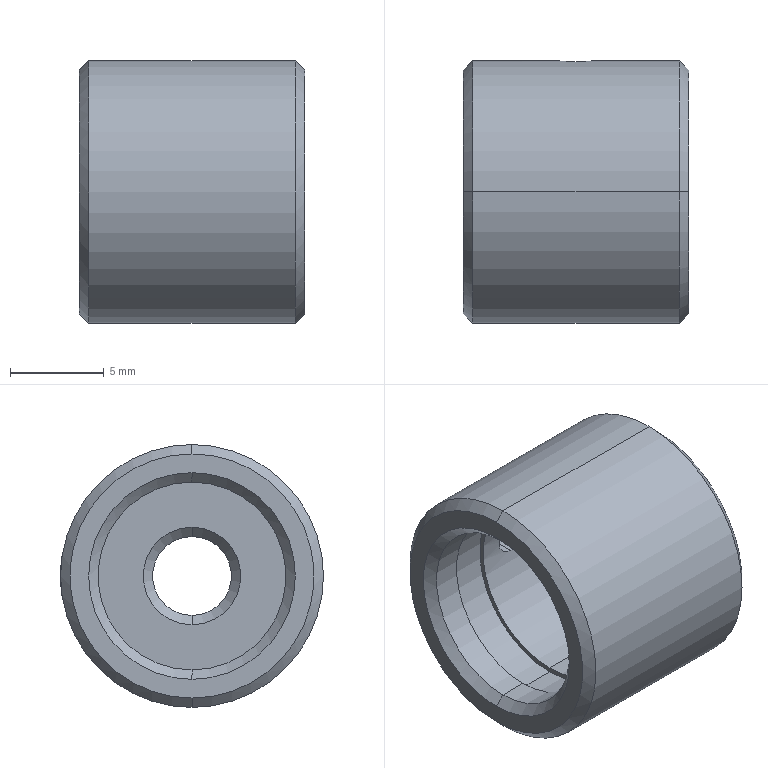Part | SolidWorks | features BaseBody 1 | 1 solid | 27 faces | box 12 x 14 x 14 mm | volume 997.34 mm3 | cylinder 12 | cone 10 | plane 5 | commonest cylinder face diameters 10 x4 1.6 x2 4.2 x2 10.5 x2 14 x2
STEP:
#1=CARTESIAN_POINT('',(-6.,6.934,0.959));
#2=VERTEX_POINT('',#1);
#3=CARTESIAN_POINT('',(-6.,6.934,-0.959));
#4=VERTEX_POINT('',#3);
#5=CARTESIAN_POINT('',(-6.,6.934,0.959));
#6=CARTESIAN_POINT('',(-6.131,6.934,0.959));
#7=CARTESIAN_POINT('',(-6.259,6.937,0.9359));
#8=CARTESIAN_POINT('',(-6.503,6.949,0.844));
#9=CARTESIAN_POINT('',(-6.615,6.957,0.7765));
#10=CARTESIAN_POINT('',(-6.808,6.975,0.6024));
#11=CARTESIAN_POINT('',(-6.887,6.983,0.4966));
#12=CARTESIAN_POINT('',(-6.996,6.996,0.2614));
#13=CARTESIAN_POINT('',(-7.025,7.,0.1312));
#14=CARTESIAN_POINT('',(-7.025,7.,-0.1276));
#15=CARTESIAN_POINT('',(-6.997,6.996,-0.258));
#16=CARTESIAN_POINT('',(-6.889,6.984,-0.4943));
#17=CARTESIAN_POINT('',(-6.81,6.975,-0.6004));
#18=CARTESIAN_POINT('',(-6.519,6.949,-0.8639));
#19=CARTESIAN_POINT('',(-6.262,6.934,-0.959));
#20=CARTESIAN_POINT('',(-6.,6.934,-0.959));
#21=B_SPLINE_CURVE_WITH_KNOTS('',3,(#5,#6,#7,#8,#9,#10,#11,#12,#13,#14,#15,#16,#17,#18,#19,#20),.UNSPECIFIED.,.F.,.F.,(4,2,2,2,2,2,2,4),(0.,0.0003877,0.0007754,0.001163,0.001551,0.001938,0.002326,0.003101),.UNSPECIFIED.);
#22=EDGE_CURVE('',#2,#4,#21,.T.);
#23=ORIENTED_EDGE('',*,*,#22,.T.);
#24=CARTESIAN_POINT('',(-6.,6.934,-0.959));
#25=CARTESIAN_POINT('',(-5.869,6.934,-0.959));
#26=CARTESIAN_POINT('',(-5.741,6.937,-0.9359));
#27=CARTESIAN_POINT('',(-5.497,6.949,-0.844));
#28=CARTESIAN_POINT('',(-5.385,6.957,-0.7765));
#29=CARTESIAN_POINT('',(-5.192,6.975,-0.6024));
#30=CARTESIAN_POINT('',(-5.113,6.983,-0.4966));
#31=CARTESIAN_POINT('',(-5.004,6.996,-0.2614));
#32=CARTESIAN_POINT('',(-4.975,7.,-0.1312));
#33=CARTESIAN_POINT('',(-4.975,7.,0.1276));
#34=CARTESIAN_POINT('',(-5.003,6.996,0.258));
#35=CARTESIAN_POINT('',(-5.111,6.984,0.4943));
#36=CARTESIAN_POINT('',(-5.19,6.975,0.6004));
#37=CARTESIAN_POINT('',(-5.481,6.949,0.8639));
#38=CARTESIAN_POINT('',(-5.738,6.934,0.959));
#39=CARTESIAN_POINT('',(-6.,6.934,0.959));
#40=B_SPLINE_CURVE_WITH_KNOTS('',3,(#24,#25,#26,#27,#28,#29,#30,#31,#32,#33,#34,#35,#36,#37,#38,#39),.UNSPECIFIED.,.F.,.F.,(4,2,2,2,2,2,2,4),(0.003101,0.003489,0.003876,0.004264,0.004652,0.005039,0.005427,0.006202),.UNSPECIFIED.);
#41=EDGE_CURVE('',#4,#2,#40,.T.);
#42=ORIENTED_EDGE('',*,*,#41,.T.);
#43=EDGE_LOOP('',(#23,#42));
#44=FACE_BOUND('',#43,.T.);
#45=CARTESIAN_POINT('',(-11.5,0.,-7.));
#46=VERTEX_POINT('',#45);
#47=CARTESIAN_POINT('',(-11.5,0.,7.));
#48=VERTEX_POINT('',#47);
#49=CARTESIAN_POINT('',(-11.5,0.,0.));
#50=DIRECTION('',(1.,0.,0.));
#51=DIRECTION('',(0.,0.,-1.));
#52=AXIS2_PLACEMENT_3D('',#49,#50,#51);
#53=CIRCLE('',#52,7.);
#54=EDGE_CURVE('',#46,#48,#53,.T.);
#55=ORIENTED_EDGE('',*,*,#54,.T.);
#56=CARTESIAN_POINT('',(-0.5,0.,7.));
#57=VERTEX_POINT('',#56);
#58=CARTESIAN_POINT('',(0.,0.,7.));
#59=DIRECTION('',(1.,0.,0.));
#60=VECTOR('',#59,1000.);
#61=LINE('',#58,#60);
#62=EDGE_CURVE('',#48,#57,#61,.T.);
#63=ORIENTED_EDGE('',*,*,#62,.T.);
#64=CARTESIAN_POINT('',(-0.5,0.,-7.));
#65=VERTEX_POINT('',#64);
#66=CARTESIAN_POINT('',(-0.5,0.,0.));
#67=DIRECTION('',(-1.,0.,0.));
#68=DIRECTION('',(0.,0.,-1.));
#69=AXIS2_PLACEMENT_3D('',#66,#67,#68);
#70=CIRCLE('',#69,7.);
#71=EDGE_CURVE('',#57,#65,#70,.T.);
#72=ORIENTED_EDGE('',*,*,#71,.T.);
#73=CARTESIAN_POINT('',(0.,0.,-7.));
#74=DIRECTION('',(1.,0.,0.));
#75=VECTOR('',#74,1000.);
#76=LINE('',#73,#75);
#77=EDGE_CURVE('',#46,#65,#76,.T.);
#78=ORIENTED_EDGE('',*,*,#77,.F.);
#79=EDGE_LOOP('',(#55,#63,#72,#78));
#80=FACE_OUTER_BOUND('',#79,.T.);
#81=CARTESIAN_POINT('',(0.,0.,0.));
#82=DIRECTION('',(1.,0.,0.));
#83=DIRECTION('',(0.,0.,-1.));
#84=AXIS2_PLACEMENT_3D('',#81,#82,#83);
#85=CYLINDRICAL_SURFACE('',#84,7.);
#86=ADVANCED_FACE('',(#44,#80),#85,.T.);
#87=CARTESIAN_POINT('',(0.,0.,6.5));
#88=VERTEX_POINT('',#87);
#89=CARTESIAN_POINT('',(0.,0.,-6.5));
#90=VERTEX_POINT('',#89);
#91=CARTESIAN_POINT('',(0.,0.,0.));
#92=DIRECTION('',(-1.,0.,0.));
#93=DIRECTION('',(0.,0.,1.));
#94=AXIS2_PLACEMENT_3D('',#91,#92,#93);
#95=CIRCLE('',#94,6.5);
#96=EDGE_CURVE('',#88,#90,#95,.T.);
#97=ORIENTED_EDGE('',*,*,#96,.T.);
#98=CARTESIAN_POINT('',(-0.5,0.,-7.));
#99=DIRECTION('',(-0.7071,0.,-0.7071));
#100=VECTOR('',#99,1000.);
#101=LINE('',#98,#100);
#102=EDGE_CURVE('',#90,#65,#101,.T.);
#103=ORIENTED_EDGE('',*,*,#102,.T.);
#104=ORIENTED_EDGE('',*,*,#71,.F.);
#105=CARTESIAN_POINT('',(-0.5,0.,7.));
#106=DIRECTION('',(-0.7071,0.,0.7071));
#107=VECTOR('',#106,1000.);
#108=LINE('',#105,#107);
#109=EDGE_CURVE('',#88,#57,#108,.T.);
#110=ORIENTED_EDGE('',*,*,#109,.F.);
#111=EDGE_LOOP('',(#97,#103,#104,#110));
#112=FACE_OUTER_BOUND('',#111,.T.);
#113=CARTESIAN_POINT('',(-0.5,0.,0.));
#114=DIRECTION('',(-1.,0.,0.));
#115=DIRECTION('',(0.,0.,1.));
#116=AXIS2_PLACEMENT_3D('',#113,#114,#115);
#117=CONICAL_SURFACE('',#116,7.,0.7854);
#118=ADVANCED_FACE('',(#112),#117,.T.);
#119=CARTESIAN_POINT('',(-12.,0.,-6.5));
#120=VERTEX_POINT('',#119);
#121=CARTESIAN_POINT('',(-12.,0.,6.5));
#122=VERTEX_POINT('',#121);
#123=CARTESIAN_POINT('',(-12.,0.,0.));
#124=DIRECTION('',(1.,0.,0.));
#125=DIRECTION('',(0.,0.,-1.));
#126=AXIS2_PLACEMENT_3D('',#123,#124,#125);
#127=CIRCLE('',#126,6.5);
#128=EDGE_CURVE('',#120,#122,#127,.T.);
#129=ORIENTED_EDGE('',*,*,#128,.T.);
#130=CARTESIAN_POINT('',(-11.5,0.,7.));
#131=DIRECTION('',(0.7071,0.,0.7071));
#132=VECTOR('',#131,1000.);
#133=LINE('',#130,#132);
#134=EDGE_CURVE('',#122,#48,#133,.T.);
#135=ORIENTED_EDGE('',*,*,#134,.T.);
#136=ORIENTED_EDGE('',*,*,#54,.F.);
#137=CARTESIAN_POINT('',(-11.5,0.,-7.));
#138=DIRECTION('',(0.7071,0.,-0.7071));
#139=VECTOR('',#138,1000.);
#140=LINE('',#137,#139);
#141=EDGE_CURVE('',#120,#46,#140,.T.);
#142=ORIENTED_EDGE('',*,*,#141,.F.);
#143=EDGE_LOOP('',(#129,#135,#136,#142));
#144=FACE_OUTER_BOUND('',#143,.T.);
#145=CARTESIAN_POINT('',(-11.5,0.,0.));
#146=DIRECTION('',(1.,0.,0.));
#147=DIRECTION('',(0.,0.,-1.));
#148=AXIS2_PLACEMENT_3D('',#145,#146,#147);
#149=CONICAL_SURFACE('',#148,7.,0.7854);
#150=ADVANCED_FACE('',(#144),#149,.T.);
#151=CARTESIAN_POINT('',(-6.,6.775,-0.8));
#152=VERTEX_POINT('',#151);
#153=CARTESIAN_POINT('',(-6.,6.775,0.8));
#154=VERTEX_POINT('',#153);
#155=CARTESIAN_POINT('',(-6.,6.775,0.));
#156=DIRECTION('',(0.,1.,0.));
#157=DIRECTION('',(0.,0.,1.));
#158=AXIS2_PLACEMENT_3D('',#155,#156,#157);
#159=CIRCLE('',#158,0.8);
#160=EDGE_CURVE('',#152,#154,#159,.T.);
#161=ORIENTED_EDGE('',*,*,#160,.F.);
#162=CARTESIAN_POINT('',(-6.,7.001,-1.026));
#163=DIRECTION('',(0.,0.7071,-0.7071));
#164=VECTOR('',#163,1000.);
#165=LINE('',#162,#164);
#166=EDGE_CURVE('',#152,#4,#165,.T.);
#167=ORIENTED_EDGE('',*,*,#166,.T.);
#168=ORIENTED_EDGE('',*,*,#22,.F.);
#169=CARTESIAN_POINT('',(-6.,7.001,1.026));
#170=DIRECTION('',(0.,0.7071,0.7071));
#171=VECTOR('',#170,1000.);
#172=LINE('',#169,#171);
#173=EDGE_CURVE('',#154,#2,#172,.T.);
#174=ORIENTED_EDGE('',*,*,#173,.F.);
#175=EDGE_LOOP('',(#161,#167,#168,#174));
#176=FACE_OUTER_BOUND('',#175,.T.);
#177=CARTESIAN_POINT('',(-6.,7.001,0.));
#178=DIRECTION('',(0.,1.,0.));
#179=DIRECTION('',(0.,0.,1.));
#180=AXIS2_PLACEMENT_3D('',#177,#178,#179);
#181=CONICAL_SURFACE('',#180,1.026,0.7854);
#182=ADVANCED_FACE('',(#176),#181,.F.);
#183=CARTESIAN_POINT('',(-1.5,0.,2.1));
#184=VERTEX_POINT('',#183);
#185=CARTESIAN_POINT('',(-1.5,0.,-2.1));
#186=VERTEX_POINT('',#185);
#187=CARTESIAN_POINT('',(-1.5,0.,0.));
#188=DIRECTION('',(1.,0.,0.));
#189=DIRECTION('',(0.,0.,-1.));
#190=AXIS2_PLACEMENT_3D('',#187,#188,#189);
#191=CIRCLE('',#190,2.1);
#192=EDGE_CURVE('',#184,#186,#191,.T.);
#193=ORIENTED_EDGE('',*,*,#192,.F.);
#194=CARTESIAN_POINT('',(0.,0.,2.1));
#195=VERTEX_POINT('',#194);
#196=CARTESIAN_POINT('',(0.,0.,2.1));
#197=DIRECTION('',(1.,0.,0.));
#198=VECTOR('',#197,1000.);
#199=LINE('',#196,#198);
#200=EDGE_CURVE('',#184,#195,#199,.T.);
#201=ORIENTED_EDGE('',*,*,#200,.T.);
#202=CARTESIAN_POINT('',(0.,0.,-2.1));
#203=VERTEX_POINT('',#202);
#204=CARTESIAN_POINT('',(0.,0.,0.));
#205=DIRECTION('',(-1.,0.,0.));
#206=DIRECTION('',(0.,0.,-1.));
#207=AXIS2_PLACEMENT_3D('',#204,#205,#206);
#208=CIRCLE('',#207,2.1);
#209=EDGE_CURVE('',#203,#195,#208,.T.);
#210=ORIENTED_EDGE('',*,*,#209,.F.);
#211=CARTESIAN_POINT('',(0.,0.,-2.1));
#212=DIRECTION('',(1.,0.,0.));
#213=VECTOR('',#212,1000.);
#214=LINE('',#211,#213);
#215=EDGE_CURVE('',#186,#203,#214,.T.);
#216=ORIENTED_EDGE('',*,*,#215,.F.);
#217=EDGE_LOOP('',(#193,#201,#210,#216));
#218=FACE_OUTER_BOUND('',#217,.T.);
#219=CARTESIAN_POINT('',(0.,0.,0.));
#220=DIRECTION('',(1.,0.,0.));
#221=DIRECTION('',(0.,0.,-1.));
#222=AXIS2_PLACEMENT_3D('',#219,#220,#221);
#223=CYLINDRICAL_SURFACE('',#222,2.1);
#224=ADVANCED_FACE('',(#218),#223,.F.);
#225=CARTESIAN_POINT('',(-6.,4.936,-0.8));
#226=VERTEX_POINT('',#225);
#227=CARTESIAN_POINT('',(-6.,4.936,0.8));
#228=VERTEX_POINT('',#227);
#229=CARTESIAN_POINT('',(-6.,4.936,-0.8));
#230=CARTESIAN_POINT('',(-6.106,4.936,-0.8));
#231=CARTESIAN_POINT('',(-6.21,4.939,-0.7791));
#232=CARTESIAN_POINT('',(-6.403,4.951,-0.6988));
#233=CARTESIAN_POINT('',(-6.492,4.96,-0.6393));
#234=CARTESIAN_POINT('',(-6.639,4.976,-0.492));
#235=CARTESIAN_POINT('',(-6.699,4.985,-0.4029));
#236=CARTESIAN_POINT('',(-6.779,4.996,-0.2105));
#237=CARTESIAN_POINT('',(-6.8,5.,-0.1051));
#238=CARTESIAN_POINT('',(-6.8,5.,0.1039));
#239=CARTESIAN_POINT('',(-6.779,4.997,0.2088));
#240=CARTESIAN_POINT('',(-6.699,4.985,0.4027));
#241=CARTESIAN_POINT('',(-6.64,4.976,0.4908));
#242=CARTESIAN_POINT('',(-6.417,4.951,0.7145));
#243=CARTESIAN_POINT('',(-6.212,4.936,0.8));
#244=CARTESIAN_POINT('',(-6.,4.936,0.8));
#245=B_SPLINE_CURVE_WITH_KNOTS('',3,(#229,#230,#231,#232,#233,#234,#235,#236,#237,#238,#239,#240,#241,#242,#243,#244),.UNSPECIFIED.,.F.,.F.,(4,2,2,2,2,2,2,4),(0.,0.0003131,0.0006261,0.0009392,0.001252,0.001565,0.001878,0.002505),.UNSPECIFIED.);
#246=EDGE_CURVE('',#226,#228,#245,.T.);
#247=ORIENTED_EDGE('',*,*,#246,.F.);
#248=CARTESIAN_POINT('',(-6.,7.,-0.8));
#249=DIRECTION('',(0.,1.,0.));
#250=VECTOR('',#249,1000.);
#251=LINE('',#248,#250);
#252=EDGE_CURVE('',#226,#152,#251,.T.);
#253=ORIENTED_EDGE('',*,*,#252,.T.);
#254=ORIENTED_EDGE('',*,*,#160,.T.);
#255=CARTESIAN_POINT('',(-6.,7.,0.8));
#256=DIRECTION('',(0.,1.,0.));
#257=VECTOR('',#256,1000.);
#258=LINE('',#255,#257);
#259=EDGE_CURVE('',#228,#154,#258,.T.);
#260=ORIENTED_EDGE('',*,*,#259,.F.);
#261=EDGE_LOOP('',(#247,#253,#254,#260));
#262=FACE_OUTER_BOUND('',#261,.T.);
#263=CARTESIAN_POINT('',(-6.,7.,0.));
#264=DIRECTION('',(0.,1.,0.));
#265=DIRECTION('',(0.,0.,1.));
#266=AXIS2_PLACEMENT_3D('',#263,#264,#265);
#267=CYLINDRICAL_SURFACE('',#266,0.8);
#268=ADVANCED_FACE('',(#262),#267,.F.);
#269=CARTESIAN_POINT('',(-11.5,0.,-5.));
#270=VERTEX_POINT('',#269);
#271=CARTESIAN_POINT('',(-11.5,0.,5.));
#272=VERTEX_POINT('',#271);
#273=CARTESIAN_POINT('',(-11.5,0.,0.));
#274=DIRECTION('',(-1.,0.,0.));
#275=DIRECTION('',(0.,0.,1.));
#276=AXIS2_PLACEMENT_3D('',#273,#274,#275);
#277=CIRCLE('',#276,5.);
#278=EDGE_CURVE('',#270,#272,#277,.T.);
#279=ORIENTED_EDGE('',*,*,#278,.F.);
#280=CARTESIAN_POINT('',(-12.,0.,-5.5));
#281=VERTEX_POINT('',#280);
#282=CARTESIAN_POINT('',(-12.,0.,-5.5));
#283=DIRECTION('',(-0.7071,0.,-0.7071));
#284=VECTOR('',#283,1000.);
#285=LINE('',#282,#284);
#286=EDGE_CURVE('',#270,#281,#285,.T.);
#287=ORIENTED_EDGE('',*,*,#286,.T.);
#288=CARTESIAN_POINT('',(-12.,0.,5.5));
#289=VERTEX_POINT('',#288);
#290=CARTESIAN_POINT('',(-12.,0.,0.));
#291=DIRECTION('',(1.,0.,0.));
#292=DIRECTION('',(0.,0.,1.));
#293=AXIS2_PLACEMENT_3D('',#290,#291,#292);
#294=CIRCLE('',#293,5.5);
#295=EDGE_CURVE('',#289,#281,#294,.T.);
#296=ORIENTED_EDGE('',*,*,#295,.F.);
#297=CARTESIAN_POINT('',(-12.,0.,5.5));
#298=DIRECTION('',(-0.7071,0.,0.7071));
#299=VECTOR('',#298,1000.);
#300=LINE('',#297,#299);
#301=EDGE_CURVE('',#272,#289,#300,.T.);
#302=ORIENTED_EDGE('',*,*,#301,.F.);
#303=EDGE_LOOP('',(#279,#287,#296,#302));
#304=FACE_OUTER_BOUND('',#303,.T.);
#305=CARTESIAN_POINT('',(-12.,0.,0.));
#306=DIRECTION('',(-1.,0.,0.));
#307=DIRECTION('',(0.,0.,1.));
#308=AXIS2_PLACEMENT_3D('',#305,#306,#307);
#309=CONICAL_SURFACE('',#308,5.5,0.7854);
#310=ADVANCED_FACE('',(#304),#309,.F.);
#311=ORIENTED_EDGE('',*,*,#192,.T.);
#312=CARTESIAN_POINT('',(-2.,0.,-2.6));
#313=VERTEX_POINT('',#312);
#314=CARTESIAN_POINT('',(-2.,0.,-2.6));
#315=DIRECTION('',(-0.7071,0.,-0.7071));
#316=VECTOR('',#315,1000.);
#317=LINE('',#314,#316);
#318=EDGE_CURVE('',#186,#313,#317,.T.);
#319=ORIENTED_EDGE('',*,*,#318,.T.);
#320=CARTESIAN_POINT('',(-2.,0.,2.6));
#321=VERTEX_POINT('',#320);
#322=CARTESIAN_POINT('',(-2.,0.,0.));
#323=DIRECTION('',(1.,0.,0.));
#324=DIRECTION('',(0.,0.,1.));
#325=AXIS2_PLACEMENT_3D('',#322,#323,#324);
#326=CIRCLE('',#325,2.6);
#327=EDGE_CURVE('',#321,#313,#326,.T.);
#328=ORIENTED_EDGE('',*,*,#327,.F.);
#329=CARTESIAN_POINT('',(-2.,0.,2.6));
#330=DIRECTION('',(-0.7071,0.,0.7071));
#331=VECTOR('',#330,1000.);
#332=LINE('',#329,#331);
#333=EDGE_CURVE('',#184,#321,#332,.T.);
#334=ORIENTED_EDGE('',*,*,#333,.F.);
#335=EDGE_LOOP('',(#311,#319,#328,#334));
#336=FACE_OUTER_BOUND('',#335,.T.);
#337=CARTESIAN_POINT('',(-2.,0.,0.));
#338=DIRECTION('',(-1.,0.,0.));
#339=DIRECTION('',(0.,0.,1.));
#340=AXIS2_PLACEMENT_3D('',#337,#338,#339);
#341=CONICAL_SURFACE('',#340,2.6,0.7854);
#342=ADVANCED_FACE('',(#336),#341,.F.);
#343=CARTESIAN_POINT('',(-8.,0.,5.));
#344=VERTEX_POINT('',#343);
#345=CARTESIAN_POINT('',(-8.,0.,-5.));
#346=VERTEX_POINT('',#345);
#347=CARTESIAN_POINT('',(-8.,0.,0.));
#348=DIRECTION('',(1.,0.,0.));
#349=DIRECTION('',(0.,0.,-1.));
#350=AXIS2_PLACEMENT_3D('',#347,#348,#349);
#351=CIRCLE('',#350,5.);
#352=EDGE_CURVE('',#344,#346,#351,.T.);
#353=ORIENTED_EDGE('',*,*,#352,.F.);
#354=CARTESIAN_POINT('',(-2.,0.,5.));
#355=VERTEX_POINT('',#354);
#356=CARTESIAN_POINT('',(0.,0.,5.));
#357=DIRECTION('',(1.,0.,0.));
#358=VECTOR('',#357,1000.);
#359=LINE('',#356,#358);
#360=EDGE_CURVE('',#344,#355,#359,.T.);
#361=ORIENTED_EDGE('',*,*,#360,.T.);
#362=CARTESIAN_POINT('',(-2.,0.,-5.));
#363=VERTEX_POINT('',#362);
#364=CARTESIAN_POINT('',(-2.,0.,0.));
#365=DIRECTION('',(-1.,0.,0.));
#366=DIRECTION('',(0.,0.,-1.));
#367=AXIS2_PLACEMENT_3D('',#364,#365,#366);
#368=CIRCLE('',#367,5.);
#369=EDGE_CURVE('',#363,#355,#368,.T.);
#370=ORIENTED_EDGE('',*,*,#369,.F.);
#371=CARTESIAN_POINT('',(0.,0.,-5.));
#372=DIRECTION('',(1.,0.,0.));
#373=VECTOR('',#372,1000.);
#374=LINE('',#371,#373);
#375=EDGE_CURVE('',#346,#363,#374,.T.);
#376=ORIENTED_EDGE('',*,*,#375,.F.);
#377=EDGE_LOOP('',(#353,#361,#370,#376));
#378=FACE_OUTER_BOUND('',#377,.T.);
#379=CARTESIAN_POINT('',(0.,0.,0.));
#380=DIRECTION('',(1.,0.,0.));
#381=DIRECTION('',(0.,0.,-1.));
#382=AXIS2_PLACEMENT_3D('',#379,#380,#381);
#383=CYLINDRICAL_SURFACE('',#382,5.);
#384=ADVANCED_FACE('',(#378),#383,.F.);
#385=ORIENTED_EDGE('',*,*,#278,.T.);
#386=CARTESIAN_POINT('',(-10.,0.,5.));
#387=VERTEX_POINT('',#386);
#388=CARTESIAN_POINT('',(0.,0.,5.));
#389=DIRECTION('',(1.,0.,0.));
#390=VECTOR('',#389,1000.);
#391=LINE('',#388,#390);
#392=EDGE_CURVE('',#272,#387,#391,.T.);
#393=ORIENTED_EDGE('',*,*,#392,.T.);
#394=CARTESIAN_POINT('',(-10.,0.,-5.));
#395=VERTEX_POINT('',#394);
#396=CARTESIAN_POINT('',(-10.,0.,0.));
#397=DIRECTION('',(-1.,0.,0.));
#398=DIRECTION('',(0.,0.,-1.));
#399=AXIS2_PLACEMENT_3D('',#396,#397,#398);
#400=CIRCLE('',#399,5.);
#401=EDGE_CURVE('',#395,#387,#400,.T.);
#402=ORIENTED_EDGE('',*,*,#401,.F.);
#403=CARTESIAN_POINT('',(0.,0.,-5.));
#404=DIRECTION('',(1.,0.,0.));
#405=VECTOR('',#404,1000.);
#406=LINE('',#403,#405);
#407=EDGE_CURVE('',#270,#395,#406,.T.);
#408=ORIENTED_EDGE('',*,*,#407,.F.);
#409=EDGE_LOOP('',(#385,#393,#402,#408));
#410=FACE_OUTER_BOUND('',#409,.T.);
#411=CARTESIAN_POINT('',(0.,0.,0.));
#412=DIRECTION('',(1.,0.,0.));
#413=DIRECTION('',(0.,0.,-1.));
#414=AXIS2_PLACEMENT_3D('',#411,#412,#413);
#415=CYLINDRICAL_SURFACE('',#414,5.);
#416=ADVANCED_FACE('',(#410),#415,.F.);
#417=CARTESIAN_POINT('',(-10.,0.,5.25));
#418=VERTEX_POINT('',#417);
#419=CARTESIAN_POINT('',(-10.,0.,-5.25));
#420=VERTEX_POINT('',#419);
#421=CARTESIAN_POINT('',(-10.,0.,0.));
#422=DIRECTION('',(1.,0.,0.));
#423=DIRECTION('',(0.,0.,-1.));
#424=AXIS2_PLACEMENT_3D('',#421,#422,#423);
#425=CIRCLE('',#424,5.25);
#426=EDGE_CURVE('',#418,#420,#425,.T.);
#427=ORIENTED_EDGE('',*,*,#426,.F.);
#428=CARTESIAN_POINT('',(-8.,0.,5.25));
#429=VERTEX_POINT('',#428);
#430=CARTESIAN_POINT('',(0.,0.,5.25));
#431=DIRECTION('',(1.,0.,0.));
#432=VECTOR('',#431,1000.);
#433=LINE('',#430,#432);
#434=EDGE_CURVE('',#418,#429,#433,.T.);
#435=ORIENTED_EDGE('',*,*,#434,.T.);
#436=CARTESIAN_POINT('',(-8.,0.,-5.25));
#437=VERTEX_POINT('',#436);
#438=CARTESIAN_POINT('',(-8.,0.,0.));
#439=DIRECTION('',(-1.,0.,0.));
#440=DIRECTION('',(0.,0.,-1.));
#441=AXIS2_PLACEMENT_3D('',#438,#439,#440);
#442=CIRCLE('',#441,5.25);
#443=EDGE_CURVE('',#437,#429,#442,.T.);
#444=ORIENTED_EDGE('',*,*,#443,.F.);
#445=CARTESIAN_POINT('',(0.,0.,-5.25));
#446=DIRECTION('',(1.,0.,0.));
#447=VECTOR('',#446,1000.);
#448=LINE('',#445,#447);
#449=EDGE_CURVE('',#420,#437,#448,.T.);
#450=ORIENTED_EDGE('',*,*,#449,.F.);
#451=EDGE_LOOP('',(#427,#435,#444,#450));
#452=FACE_OUTER_BOUND('',#451,.T.);
#453=CARTESIAN_POINT('',(0.,0.,0.));
#454=DIRECTION('',(1.,0.,0.));
#455=DIRECTION('',(0.,0.,-1.));
#456=AXIS2_PLACEMENT_3D('',#453,#454,#455);
#457=CYLINDRICAL_SURFACE('',#456,5.25);
#458=ADVANCED_FACE('',(#452),#457,.F.);
#459=ORIENTED_EDGE('',*,*,#62,.F.);
#460=CARTESIAN_POINT('',(-11.5,0.,0.));
#461=DIRECTION('',(1.,0.,0.));
#462=DIRECTION('',(0.,0.,-1.));
#463=AXIS2_PLACEMENT_3D('',#460,#461,#462);
#464=CIRCLE('',#463,7.);
#465=EDGE_CURVE('',#48,#46,#464,.T.);
#466=ORIENTED_EDGE('',*,*,#465,.T.);
#467=ORIENTED_EDGE('',*,*,#77,.T.);
#468=CARTESIAN_POINT('',(-0.5,0.,0.));
#469=DIRECTION('',(-1.,0.,0.));
#470=DIRECTION('',(0.,0.,-1.));
#471=AXIS2_PLACEMENT_3D('',#468,#469,#470);
#472=CIRCLE('',#471,7.);
#473=EDGE_CURVE('',#65,#57,#472,.T.);
#474=ORIENTED_EDGE('',*,*,#473,.T.);
#475=EDGE_LOOP('',(#459,#466,#467,#474));
#476=FACE_OUTER_BOUND('',#475,.T.);
#477=CARTESIAN_POINT('',(0.,0.,0.));
#478=DIRECTION('',(1.,0.,0.));
#479=DIRECTION('',(0.,0.,-1.));
#480=AXIS2_PLACEMENT_3D('',#477,#478,#479);
#481=CYLINDRICAL_SURFACE('',#480,7.);
#482=ADVANCED_FACE('',(#476),#481,.T.);
#483=ORIENTED_EDGE('',*,*,#102,.F.);
#484=CARTESIAN_POINT('',(0.,0.,0.));
#485=DIRECTION('',(-1.,0.,0.));
#486=DIRECTION('',(0.,0.,1.));
#487=AXIS2_PLACEMENT_3D('',#484,#485,#486);
#488=CIRCLE('',#487,6.5);
#489=EDGE_CURVE('',#90,#88,#488,.T.);
#490=ORIENTED_EDGE('',*,*,#489,.T.);
#491=ORIENTED_EDGE('',*,*,#109,.T.);
#492=ORIENTED_EDGE('',*,*,#473,.F.);
#493=EDGE_LOOP('',(#483,#490,#491,#492));
#494=FACE_OUTER_BOUND('',#493,.T.);
#495=CARTESIAN_POINT('',(-0.5,0.,0.));
#496=DIRECTION('',(-1.,0.,0.));
#497=DIRECTION('',(0.,0.,1.));
#498=AXIS2_PLACEMENT_3D('',#495,#496,#497);
#499=CONICAL_SURFACE('',#498,7.,0.7854);
#500=ADVANCED_FACE('',(#494),#499,.T.);
#501=ORIENTED_EDGE('',*,*,#134,.F.);
#502=CARTESIAN_POINT('',(-12.,0.,0.));
#503=DIRECTION('',(1.,0.,0.));
#504=DIRECTION('',(0.,0.,-1.));
#505=AXIS2_PLACEMENT_3D('',#502,#503,#504);
#506=CIRCLE('',#505,6.5);
#507=EDGE_CURVE('',#122,#120,#506,.T.);
#508=ORIENTED_EDGE('',*,*,#507,.T.);
#509=ORIENTED_EDGE('',*,*,#141,.T.);
#510=ORIENTED_EDGE('',*,*,#465,.F.);
#511=EDGE_LOOP('',(#501,#508,#509,#510));
#512=FACE_OUTER_BOUND('',#511,.T.);
#513=CARTESIAN_POINT('',(-11.5,0.,0.));
#514=DIRECTION('',(1.,0.,0.));
#515=DIRECTION('',(0.,0.,-1.));
#516=AXIS2_PLACEMENT_3D('',#513,#514,#515);
#517=CONICAL_SURFACE('',#516,7.,0.7854);
#518=ADVANCED_FACE('',(#512),#517,.T.);
#519=ORIENTED_EDGE('',*,*,#209,.T.);
#520=CARTESIAN_POINT('',(0.,0.,0.));
#521=DIRECTION('',(-1.,0.,0.));
#522=DIRECTION('',(0.,0.,-1.));
#523=AXIS2_PLACEMENT_3D('',#520,#521,#522);
#524=CIRCLE('',#523,2.1);
#525=EDGE_CURVE('',#195,#203,#524,.T.);
#526=ORIENTED_EDGE('',*,*,#525,.T.);
#527=EDGE_LOOP('',(#519,#526));
#528=FACE_BOUND('',#527,.T.);
#529=ORIENTED_EDGE('',*,*,#96,.F.);
#530=ORIENTED_EDGE('',*,*,#489,.F.);
#531=EDGE_LOOP('',(#529,#530));
#532=FACE_OUTER_BOUND('',#531,.T.);
#533=CARTESIAN_POINT('',(0.,2.1,0.));
#534=DIRECTION('',(1.,0.,0.));
#535=DIRECTION('',(0.,0.,-1.));
#536=AXIS2_PLACEMENT_3D('',#533,#534,#535);
#537=PLANE('',#536);
#538=ADVANCED_FACE('',(#528,#532),#537,.T.);
#539=ORIENTED_EDGE('',*,*,#166,.F.);
#540=CARTESIAN_POINT('',(-6.,6.775,0.));
#541=DIRECTION('',(0.,1.,0.));
#542=DIRECTION('',(0.,0.,1.));
#543=AXIS2_PLACEMENT_3D('',#540,#541,#542);
#544=CIRCLE('',#543,0.8);
#545=EDGE_CURVE('',#154,#152,#544,.T.);
#546=ORIENTED_EDGE('',*,*,#545,.F.);
#547=ORIENTED_EDGE('',*,*,#173,.T.);
#548=ORIENTED_EDGE('',*,*,#41,.F.);
#549=EDGE_LOOP('',(#539,#546,#547,#548));
#550=FACE_OUTER_BOUND('',#549,.T.);
#551=CARTESIAN_POINT('',(-6.,7.001,0.));
#552=DIRECTION('',(0.,1.,0.));
#553=DIRECTION('',(0.,0.,1.));
#554=AXIS2_PLACEMENT_3D('',#551,#552,#553);
#555=CONICAL_SURFACE('',#554,1.026,0.7854);
#556=ADVANCED_FACE('',(#550),#555,.F.);
#557=ORIENTED_EDGE('',*,*,#128,.F.);
#558=ORIENTED_EDGE('',*,*,#507,.F.);
#559=EDGE_LOOP('',(#557,#558));
#560=FACE_OUTER_BOUND('',#559,.T.);
#561=ORIENTED_EDGE('',*,*,#295,.T.);
#562=CARTESIAN_POINT('',(-12.,0.,0.));
#563=DIRECTION('',(1.,0.,0.));
#564=DIRECTION('',(0.,0.,1.));
#565=AXIS2_PLACEMENT_3D('',#562,#563,#564);
#566=CIRCLE('',#565,5.5);
#567=EDGE_CURVE('',#281,#289,#566,.T.);
#568=ORIENTED_EDGE('',*,*,#567,.T.);
#569=EDGE_LOOP('',(#561,#568));
#570=FACE_BOUND('',#569,.T.);
#571=CARTESIAN_POINT('',(-12.,7.,0.));
#572=DIRECTION('',(-1.,0.,0.));
#573=DIRECTION('',(0.,0.,1.));
#574=AXIS2_PLACEMENT_3D('',#571,#572,#573);
#575=PLANE('',#574);
#576=ADVANCED_FACE('',(#560,#570),#575,.T.);
#577=ORIENTED_EDGE('',*,*,#200,.F.);
#578=CARTESIAN_POINT('',(-1.5,0.,0.));
#579=DIRECTION('',(1.,0.,0.));
#580=DIRECTION('',(0.,0.,-1.));
#581=AXIS2_PLACEMENT_3D('',#578,#579,#580);
#582=CIRCLE('',#581,2.1);
#583=EDGE_CURVE('',#186,#184,#582,.T.);
#584=ORIENTED_EDGE('',*,*,#583,.F.);
#585=ORIENTED_EDGE('',*,*,#215,.T.);
#586=ORIENTED_EDGE('',*,*,#525,.F.);
#587=EDGE_LOOP('',(#577,#584,#585,#586));
#588=FACE_OUTER_BOUND('',#587,.T.);
#589=CARTESIAN_POINT('',(0.,0.,0.));
#590=DIRECTION('',(1.,0.,0.));
#591=DIRECTION('',(0.,0.,-1.));
#592=AXIS2_PLACEMENT_3D('',#589,#590,#591);
#593=CYLINDRICAL_SURFACE('',#592,2.1);
#594=ADVANCED_FACE('',(#588),#593,.F.);
#595=ORIENTED_EDGE('',*,*,#252,.F.);
#596=CARTESIAN_POINT('',(-6.,4.936,0.8));
#597=CARTESIAN_POINT('',(-5.894,4.936,0.8));
#598=CARTESIAN_POINT('',(-5.79,4.939,0.7791));
#599=CARTESIAN_POINT('',(-5.597,4.951,0.6988));
#600=CARTESIAN_POINT('',(-5.508,4.96,0.6393));
#601=CARTESIAN_POINT('',(-5.361,4.976,0.492));
#602=CARTESIAN_POINT('',(-5.301,4.985,0.4029));
#603=CARTESIAN_POINT('',(-5.221,4.996,0.2105));
#604=CARTESIAN_POINT('',(-5.2,5.,0.1051));
#605=CARTESIAN_POINT('',(-5.2,5.,-0.1039));
#606=CARTESIAN_POINT('',(-5.221,4.997,-0.2088));
#607=CARTESIAN_POINT('',(-5.301,4.985,-0.4027));
#608=CARTESIAN_POINT('',(-5.36,4.976,-0.4908));
#609=CARTESIAN_POINT('',(-5.583,4.951,-0.7145));
#610=CARTESIAN_POINT('',(-5.788,4.936,-0.8));
#611=CARTESIAN_POINT('',(-6.,4.936,-0.8));
#612=B_SPLINE_CURVE_WITH_KNOTS('',3,(#596,#597,#598,#599,#600,#601,#602,#603,#604,#605,#606,#607,#608,#609,#610,#611),.UNSPECIFIED.,.F.,.F.,(4,2,2,2,2,2,2,4),(0.002505,0.002818,0.003131,0.003444,0.003757,0.00407,0.004383,0.005009),.UNSPECIFIED.);
#613=EDGE_CURVE('',#228,#226,#612,.T.);
#614=ORIENTED_EDGE('',*,*,#613,.F.);
#615=ORIENTED_EDGE('',*,*,#259,.T.);
#616=ORIENTED_EDGE('',*,*,#545,.T.);
#617=EDGE_LOOP('',(#595,#614,#615,#616));
#618=FACE_OUTER_BOUND('',#617,.T.);
#619=CARTESIAN_POINT('',(-6.,7.,0.));
#620=DIRECTION('',(0.,1.,0.));
#621=DIRECTION('',(0.,0.,1.));
#622=AXIS2_PLACEMENT_3D('',#619,#620,#621);
#623=CYLINDRICAL_SURFACE('',#622,0.8);
#624=ADVANCED_FACE('',(#618),#623,.F.);
#625=ORIENTED_EDGE('',*,*,#286,.F.);
#626=CARTESIAN_POINT('',(-11.5,0.,0.));
#627=DIRECTION('',(-1.,0.,0.));
#628=DIRECTION('',(0.,0.,1.));
#629=AXIS2_PLACEMENT_3D('',#626,#627,#628);
#630=CIRCLE('',#629,5.);
#631=EDGE_CURVE('',#272,#270,#630,.T.);
#632=ORIENTED_EDGE('',*,*,#631,.F.);
#633=ORIENTED_EDGE('',*,*,#301,.T.);
#634=ORIENTED_EDGE('',*,*,#567,.F.);
#635=EDGE_LOOP('',(#625,#632,#633,#634));
#636=FACE_OUTER_BOUND('',#635,.T.);
#637=CARTESIAN_POINT('',(-12.,0.,0.));
#638=DIRECTION('',(-1.,0.,0.));
#639=DIRECTION('',(0.,0.,1.));
#640=AXIS2_PLACEMENT_3D('',#637,#638,#639);
#641=CONICAL_SURFACE('',#640,5.5,0.7854);
#642=ADVANCED_FACE('',(#636),#641,.F.);
#643=ORIENTED_EDGE('',*,*,#318,.F.);
#644=ORIENTED_EDGE('',*,*,#583,.T.);
#645=ORIENTED_EDGE('',*,*,#333,.T.);
#646=CARTESIAN_POINT('',(-2.,0.,0.));
#647=DIRECTION('',(1.,0.,0.));
#648=DIRECTION('',(0.,0.,1.));
#649=AXIS2_PLACEMENT_3D('',#646,#647,#648);
#650=CIRCLE('',#649,2.6);
#651=EDGE_CURVE('',#313,#321,#650,.T.);
#652=ORIENTED_EDGE('',*,*,#651,.F.);
#653=EDGE_LOOP('',(#643,#644,#645,#652));
#654=FACE_OUTER_BOUND('',#653,.T.);
#655=CARTESIAN_POINT('',(-2.,0.,0.));
#656=DIRECTION('',(-1.,0.,0.));
#657=DIRECTION('',(0.,0.,1.));
#658=AXIS2_PLACEMENT_3D('',#655,#656,#657);
#659=CONICAL_SURFACE('',#658,2.6,0.7854);
#660=ADVANCED_FACE('',(#654),#659,.F.);
#661=ORIENTED_EDGE('',*,*,#360,.F.);
#662=CARTESIAN_POINT('',(-8.,0.,0.));
#663=DIRECTION('',(1.,0.,0.));
#664=DIRECTION('',(0.,0.,-1.));
#665=AXIS2_PLACEMENT_3D('',#662,#663,#664);
#666=CIRCLE('',#665,5.);
#667=EDGE_CURVE('',#346,#344,#666,.T.);
#668=ORIENTED_EDGE('',*,*,#667,.F.);
#669=ORIENTED_EDGE('',*,*,#375,.T.);
#670=CARTESIAN_POINT('',(-2.,0.,0.));
#671=DIRECTION('',(-1.,0.,0.));
#672=DIRECTION('',(0.,0.,-1.));
#673=AXIS2_PLACEMENT_3D('',#670,#671,#672);
#674=CIRCLE('',#673,5.);
#675=EDGE_CURVE('',#355,#363,#674,.T.);
#676=ORIENTED_EDGE('',*,*,#675,.F.);
#677=EDGE_LOOP('',(#661,#668,#669,#676));
#678=FACE_OUTER_BOUND('',#677,.T.);
#679=ORIENTED_EDGE('',*,*,#613,.T.);
#680=ORIENTED_EDGE('',*,*,#246,.T.);
#681=EDGE_LOOP('',(#679,#680));
#682=FACE_BOUND('',#681,.T.);
#683=CARTESIAN_POINT('',(0.,0.,0.));
#684=DIRECTION('',(1.,0.,0.));
#685=DIRECTION('',(0.,0.,-1.));
#686=AXIS2_PLACEMENT_3D('',#683,#684,#685);
#687=CYLINDRICAL_SURFACE('',#686,5.);
#688=ADVANCED_FACE('',(#678,#682),#687,.F.);
#689=ORIENTED_EDGE('',*,*,#392,.F.);
#690=ORIENTED_EDGE('',*,*,#631,.T.);
#691=ORIENTED_EDGE('',*,*,#407,.T.);
#692=CARTESIAN_POINT('',(-10.,0.,0.));
#693=DIRECTION('',(-1.,0.,0.));
#694=DIRECTION('',(0.,0.,-1.));
#695=AXIS2_PLACEMENT_3D('',#692,#693,#694);
#696=CIRCLE('',#695,5.);
#697=EDGE_CURVE('',#387,#395,#696,.T.);
#698=ORIENTED_EDGE('',*,*,#697,.F.);
#699=EDGE_LOOP('',(#689,#690,#691,#698));
#700=FACE_OUTER_BOUND('',#699,.T.);
#701=CARTESIAN_POINT('',(0.,0.,0.));
#702=DIRECTION('',(1.,0.,0.));
#703=DIRECTION('',(0.,0.,-1.));
#704=AXIS2_PLACEMENT_3D('',#701,#702,#703);
#705=CYLINDRICAL_SURFACE('',#704,5.);
#706=ADVANCED_FACE('',(#700),#705,.F.);
#707=ORIENTED_EDGE('',*,*,#369,.T.);
#708=ORIENTED_EDGE('',*,*,#675,.T.);
#709=EDGE_LOOP('',(#707,#708));
#710=FACE_OUTER_BOUND('',#709,.T.);
#711=ORIENTED_EDGE('',*,*,#327,.T.);
#712=ORIENTED_EDGE('',*,*,#651,.T.);
#713=EDGE_LOOP('',(#711,#712));
#714=FACE_BOUND('',#713,.T.);
#715=CARTESIAN_POINT('',(-2.,5.,0.));
#716=DIRECTION('',(-1.,0.,0.));
#717=DIRECTION('',(0.,0.,1.));
#718=AXIS2_PLACEMENT_3D('',#715,#716,#717);
#719=PLANE('',#718);
#720=ADVANCED_FACE('',(#710,#714),#719,.T.);
#721=ORIENTED_EDGE('',*,*,#443,.T.);
#722=CARTESIAN_POINT('',(-8.,0.,0.));
#723=DIRECTION('',(-1.,0.,0.));
#724=DIRECTION('',(0.,0.,-1.));
#725=AXIS2_PLACEMENT_3D('',#722,#723,#724);
#726=CIRCLE('',#725,5.25);
#727=EDGE_CURVE('',#429,#437,#726,.T.);
#728=ORIENTED_EDGE('',*,*,#727,.T.);
#729=EDGE_LOOP('',(#721,#728));
#730=FACE_OUTER_BOUND('',#729,.T.);
#731=ORIENTED_EDGE('',*,*,#667,.T.);
#732=ORIENTED_EDGE('',*,*,#352,.T.);
#733=EDGE_LOOP('',(#731,#732));
#734=FACE_BOUND('',#733,.T.);
#735=CARTESIAN_POINT('',(-8.,5.25,0.));
#736=DIRECTION('',(-1.,0.,0.));
#737=DIRECTION('',(0.,0.,1.));
#738=AXIS2_PLACEMENT_3D('',#735,#736,#737);
#739=PLANE('',#738);
#740=ADVANCED_FACE('',(#730,#734),#739,.T.);
#741=ORIENTED_EDGE('',*,*,#401,.T.);
#742=ORIENTED_EDGE('',*,*,#697,.T.);
#743=EDGE_LOOP('',(#741,#742));
#744=FACE_BOUND('',#743,.T.);
#745=CARTESIAN_POINT('',(-10.,0.,0.));
#746=DIRECTION('',(1.,0.,0.));
#747=DIRECTION('',(0.,0.,-1.));
#748=AXIS2_PLACEMENT_3D('',#745,#746,#747);
#749=CIRCLE('',#748,5.25);
#750=EDGE_CURVE('',#420,#418,#749,.T.);
#751=ORIENTED_EDGE('',*,*,#750,.T.);
#752=ORIENTED_EDGE('',*,*,#426,.T.);
#753=EDGE_LOOP('',(#751,#752));
#754=FACE_OUTER_BOUND('',#753,.T.);
#755=CARTESIAN_POINT('',(-10.,5.,0.));
#756=DIRECTION('',(1.,0.,0.));
#757=DIRECTION('',(0.,0.,-1.));
#758=AXIS2_PLACEMENT_3D('',#755,#756,#757);
#759=PLANE('',#758);
#760=ADVANCED_FACE('',(#744,#754),#759,.T.);
#761=ORIENTED_EDGE('',*,*,#434,.F.);
#762=ORIENTED_EDGE('',*,*,#750,.F.);
#763=ORIENTED_EDGE('',*,*,#449,.T.);
#764=ORIENTED_EDGE('',*,*,#727,.F.);
#765=EDGE_LOOP('',(#761,#762,#763,#764));
#766=FACE_OUTER_BOUND('',#765,.T.);
#767=CARTESIAN_POINT('',(0.,0.,0.));
#768=DIRECTION('',(1.,0.,0.));
#769=DIRECTION('',(0.,0.,-1.));
#770=AXIS2_PLACEMENT_3D('',#767,#768,#769);
#771=CYLINDRICAL_SURFACE('',#770,5.25);
#772=ADVANCED_FACE('',(#766),#771,.F.);
#773=CLOSED_SHELL('',(#86,#118,#150,#182,#224,#268,#310,#342,#384,#416,#458,#482,#500,#518,#538,#556,#576,#594,#624,#642,#660,#688,#706,#720,#740,#760,#772));
#774=MANIFOLD_SOLID_BREP('',#773);
#775=CARTESIAN_POINT('',(0.,0.,0.));
#776=DIRECTION('',(0.,0.,1.));
#777=DIRECTION('',(1.,0.,0.));
#778=AXIS2_PLACEMENT_3D('',#775,#776,#777);
#779=(LENGTH_UNIT()NAMED_UNIT(*)SI_UNIT(.MILLI.,.METRE.));
#780=UNCERTAINTY_MEASURE_WITH_UNIT(LENGTH_MEASURE(0.00001),#779,'','');
#781=(NAMED_UNIT(*)PLANE_ANGLE_UNIT()SI_UNIT($,.RADIAN.));
#782=(NAMED_UNIT(*)SI_UNIT($,.STERADIAN.)SOLID_ANGLE_UNIT());
#783=(GEOMETRIC_REPRESENTATION_CONTEXT(3)GLOBAL_UNCERTAINTY_ASSIGNED_CONTEXT((#780))GLOBAL_UNIT_ASSIGNED_CONTEXT((#779,#781,#782))REPRESENTATION_CONTEXT('',''));
#784=ADVANCED_BREP_SHAPE_REPRESENTATION('',(#774,#778),#783);